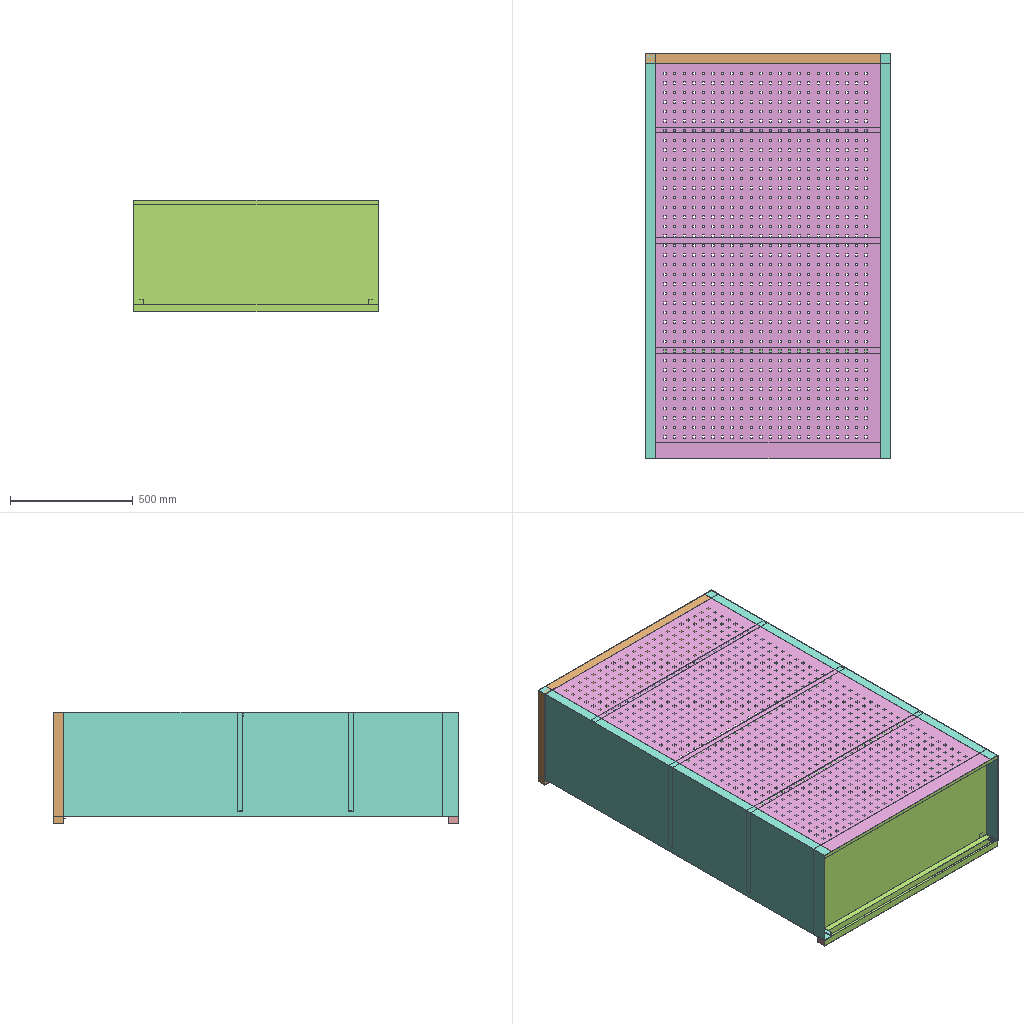Assembly | SolidWorks | 6 different items | 9 placed | box 1002 x 1650 x 455 mm
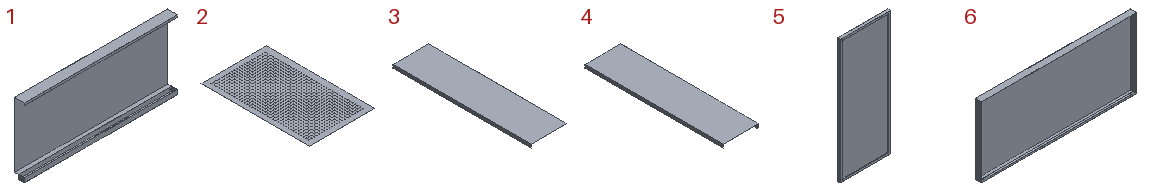Parts list (item | quantity | size | volume | features):
1 | x1 | 998 x 65 x 452 mm | 623910 mm3 | features ICE 3, ExtruThin 1
2 | x1 | - | 1559902 mm3 | features Extrusion 1, ICE 1, LPattern 1
3 | x2 | 427 x 1649 x 42 mm | 892128 mm3 | features ExtruThin 1, ICE 1
4 | x1 | 427 x 1649 x 42 mm | 892128 mm3 | features ExtruThin 1, ICE 1
5 | x3 | 401 x 23 x 992 mm | 497496 mm3 | features BossThin 2, ExtruThin 1
6 | x1 | 1002 x 50 x 455 mm | 600406 mm3 | features ICE 4, ExtruThin 1
Mates (type | each side: item.copy, entity, surface, feature):
Coincident | 1.1 face plane Extrude-Thin1 | 2.1 face plane Extrude1 | 2 times
Coincident | 1.1 face plane Extrude-Thin1 | 3.1 face plane Extrude-Thin1 | 2 times
Coincident | 2.1 face plane Extrude1 | 3.1 face plane Extrude-Thin1 | 2 times
Coincident | 2.1 face plane Extrude1 | 3.2 face plane Extrude-Thin1
Coincident | 1.1 face plane Extrude-Thin1 | 3.2 face plane Extrude-Thin1 | 2 times
Coincident | 2.1 face plane Extrude1 | 6.1 face plane Extrude-Thin1
Coincident | 3.2 face plane Extrude-Thin1 | 6.1 face plane Extrude-Thin1
Coincident | 3.2 face plane Extrude-Thin1 | 6.1 face plane Extrude3
Coincident | 3.1 face plane Extrude-Thin1 | 5.1 face plane Extrude-Thin1
Coincident | 2.1 face plane Extrude1 | 5.1 face plane Extrude-Thin1
Coincident | 5.1 face plane Extrude-Thin4 | 5.2 face plane Extrude-Thin1
Coincident | 3.2 face plane Extrude-Thin1 | 5.2 face plane Extrude-Thin1
Coincident | 5.2 face plane Extrude-Thin1 | 5.3 face plane Extrude-Thin1
Coincident | 3.2 face plane Extrude-Thin1 | 5.3 face plane Extrude-Thin1
DistanceDim | 5.2 face plane Extrude-Thin1 | 5.3 face plane Extrude-Thin1
DistanceDim | 5.1 face plane Extrude-Thin1 | 5.2 face plane Extrude-Thin1
DistanceDim | 6.1 face plane Extrude-Thin1 | 5.1 face plane Extrude-Thin1